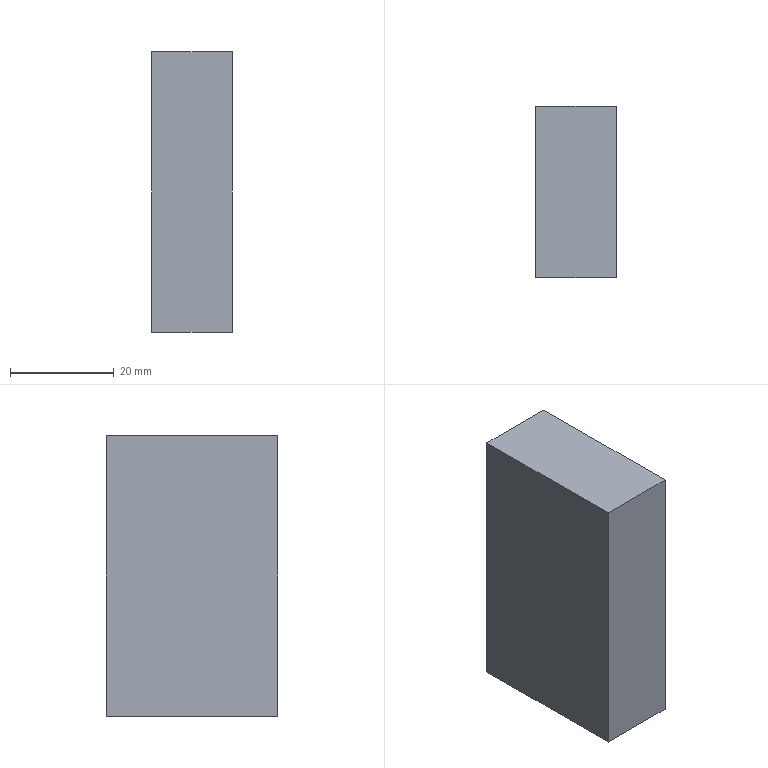Part | NX | features DATUM_CSYS 2, BLOCK 1, EXTRUDE 1, SKETCH 1 | 1 solid | 8 faces | box 15.5 x 33 x 54 mm | volume 25530 mm3 | plane 7 | cylinder 1 | commonest cylinder face diameters 22 x1
STEP:
#1=CARTESIAN_POINT('',(15.5,0.,54.));
#2=VERTEX_POINT('',#1);
#3=CARTESIAN_POINT('',(0.,0.,54.));
#4=VERTEX_POINT('',#3);
#5=CARTESIAN_POINT('',(7.75,0.,54.));
#6=DIRECTION('',(-1.,0.,0.));
#7=VECTOR('',#6,1000.);
#8=LINE('',#5,#7);
#9=EDGE_CURVE('',#2,#4,#8,.T.);
#10=ORIENTED_EDGE('',*,*,#9,.F.);
#11=CARTESIAN_POINT('',(15.5,33.,54.));
#12=VERTEX_POINT('',#11);
#13=CARTESIAN_POINT('',(15.5,16.5,54.));
#14=DIRECTION('',(0.,-1.,0.));
#15=VECTOR('',#14,1000.);
#16=LINE('',#13,#15);
#17=EDGE_CURVE('',#12,#2,#16,.T.);
#18=ORIENTED_EDGE('',*,*,#17,.F.);
#19=CARTESIAN_POINT('',(0.,33.,54.));
#20=VERTEX_POINT('',#19);
#21=CARTESIAN_POINT('',(7.75,33.,54.));
#22=DIRECTION('',(1.,0.,0.));
#23=VECTOR('',#22,1000.);
#24=LINE('',#21,#23);
#25=EDGE_CURVE('',#20,#12,#24,.T.);
#26=ORIENTED_EDGE('',*,*,#25,.F.);
#27=CARTESIAN_POINT('',(0.,16.5,54.));
#28=DIRECTION('',(0.,1.,0.));
#29=VECTOR('',#28,1000.);
#30=LINE('',#27,#29);
#31=EDGE_CURVE('',#4,#20,#30,.T.);
#32=ORIENTED_EDGE('',*,*,#31,.F.);
#33=EDGE_LOOP('',(#10,#18,#26,#32));
#34=FACE_BOUND('',#33,.T.);
#35=CARTESIAN_POINT('',(7.75,16.5,54.));
#36=DIRECTION('',(0.,0.,1.));
#37=DIRECTION('',(1.,0.,0.));
#38=AXIS2_PLACEMENT_3D('',#35,#36,#37);
#39=PLANE('',#38);
#40=ADVANCED_FACE('',(#34),#39,.T.);
#41=CARTESIAN_POINT('',(15.5,0.,0.));
#42=VERTEX_POINT('',#41);
#43=CARTESIAN_POINT('',(15.5,0.,0.));
#44=DIRECTION('',(0.,0.,1.));
#45=VECTOR('',#44,1000.);
#46=LINE('',#43,#45);
#47=EDGE_CURVE('',#42,#2,#46,.T.);
#48=ORIENTED_EDGE('',*,*,#47,.T.);
#49=ORIENTED_EDGE('',*,*,#9,.T.);
#50=CARTESIAN_POINT('',(0.,0.,0.));
#51=VERTEX_POINT('',#50);
#52=CARTESIAN_POINT('',(0.,0.,0.));
#53=DIRECTION('',(0.,0.,1.));
#54=VECTOR('',#53,1000.);
#55=LINE('',#52,#54);
#56=EDGE_CURVE('',#51,#4,#55,.T.);
#57=ORIENTED_EDGE('',*,*,#56,.F.);
#58=CARTESIAN_POINT('',(7.75,0.,0.));
#59=DIRECTION('',(1.,0.,0.));
#60=VECTOR('',#59,1000.);
#61=LINE('',#58,#60);
#62=EDGE_CURVE('',#51,#42,#61,.T.);
#63=ORIENTED_EDGE('',*,*,#62,.T.);
#64=EDGE_LOOP('',(#48,#49,#57,#63));
#65=FACE_BOUND('',#64,.T.);
#66=CARTESIAN_POINT('',(7.75,0.,0.));
#67=DIRECTION('',(0.,-1.,0.));
#68=DIRECTION('',(0.,0.,-1.));
#69=AXIS2_PLACEMENT_3D('',#66,#67,#68);
#70=PLANE('',#69);
#71=ADVANCED_FACE('',(#65),#70,.T.);
#72=ORIENTED_EDGE('',*,*,#56,.T.);
#73=ORIENTED_EDGE('',*,*,#31,.T.);
#74=CARTESIAN_POINT('',(0.,33.,0.));
#75=VERTEX_POINT('',#74);
#76=CARTESIAN_POINT('',(0.,33.,0.));
#77=DIRECTION('',(0.,0.,1.));
#78=VECTOR('',#77,1000.);
#79=LINE('',#76,#78);
#80=EDGE_CURVE('',#75,#20,#79,.T.);
#81=ORIENTED_EDGE('',*,*,#80,.F.);
#82=CARTESIAN_POINT('',(0.,16.5,0.));
#83=DIRECTION('',(0.,-1.,0.));
#84=VECTOR('',#83,1000.);
#85=LINE('',#82,#84);
#86=EDGE_CURVE('',#75,#51,#85,.T.);
#87=ORIENTED_EDGE('',*,*,#86,.T.);
#88=EDGE_LOOP('',(#72,#73,#81,#87));
#89=FACE_BOUND('',#88,.T.);
#90=CARTESIAN_POINT('',(0.,16.5,0.));
#91=DIRECTION('',(-1.,0.,0.));
#92=DIRECTION('',(0.,0.,1.));
#93=AXIS2_PLACEMENT_3D('',#90,#91,#92);
#94=PLANE('',#93);
#95=ADVANCED_FACE('',(#89),#94,.T.);
#96=ORIENTED_EDGE('',*,*,#80,.T.);
#97=ORIENTED_EDGE('',*,*,#25,.T.);
#98=CARTESIAN_POINT('',(15.5,33.,0.));
#99=VERTEX_POINT('',#98);
#100=CARTESIAN_POINT('',(15.5,33.,0.));
#101=DIRECTION('',(0.,0.,1.));
#102=VECTOR('',#101,1000.);
#103=LINE('',#100,#102);
#104=EDGE_CURVE('',#99,#12,#103,.T.);
#105=ORIENTED_EDGE('',*,*,#104,.F.);
#106=CARTESIAN_POINT('',(7.75,33.,0.));
#107=DIRECTION('',(-1.,0.,0.));
#108=VECTOR('',#107,1000.);
#109=LINE('',#106,#108);
#110=EDGE_CURVE('',#99,#75,#109,.T.);
#111=ORIENTED_EDGE('',*,*,#110,.T.);
#112=EDGE_LOOP('',(#96,#97,#105,#111));
#113=FACE_BOUND('',#112,.T.);
#114=CARTESIAN_POINT('',(7.75,33.,0.));
#115=DIRECTION('',(0.,1.,0.));
#116=DIRECTION('',(0.,0.,1.));
#117=AXIS2_PLACEMENT_3D('',#114,#115,#116);
#118=PLANE('',#117);
#119=ADVANCED_FACE('',(#113),#118,.T.);
#120=CARTESIAN_POINT('',(15.5,16.5,0.));
#121=DIRECTION('',(0.,1.,0.));
#122=VECTOR('',#121,1000.);
#123=LINE('',#120,#122);
#124=EDGE_CURVE('',#42,#99,#123,.T.);
#125=ORIENTED_EDGE('',*,*,#124,.F.);
#126=ORIENTED_EDGE('',*,*,#62,.F.);
#127=ORIENTED_EDGE('',*,*,#86,.F.);
#128=ORIENTED_EDGE('',*,*,#110,.F.);
#129=EDGE_LOOP('',(#125,#126,#127,#128));
#130=FACE_BOUND('',#129,.T.);
#131=CARTESIAN_POINT('',(7.75,16.5,0.));
#132=DIRECTION('',(0.,0.,-1.));
#133=DIRECTION('',(-1.,0.,0.));
#134=AXIS2_PLACEMENT_3D('',#131,#132,#133);
#135=PLANE('',#134);
#136=ADVANCED_FACE('',(#130),#135,.T.);
#137=CARTESIAN_POINT('',(15.5,30.,27.));
#138=VERTEX_POINT('',#137);
#139=CARTESIAN_POINT('',(15.5,19.,27.));
#140=DIRECTION('',(1.,0.,0.));
#141=DIRECTION('',(0.,1.,0.));
#142=AXIS2_PLACEMENT_3D('',#139,#140,#141);
#143=CIRCLE('',#142,11.);
#144=EDGE_CURVE('',#138,#138,#143,.T.);
#145=ORIENTED_EDGE('',*,*,#144,.F.);
#146=EDGE_LOOP('',(#145));
#147=FACE_BOUND('',#146,.T.);
#148=ORIENTED_EDGE('',*,*,#124,.T.);
#149=ORIENTED_EDGE('',*,*,#104,.T.);
#150=ORIENTED_EDGE('',*,*,#17,.T.);
#151=ORIENTED_EDGE('',*,*,#47,.F.);
#152=EDGE_LOOP('',(#148,#149,#150,#151));
#153=FACE_BOUND('',#152,.T.);
#154=CARTESIAN_POINT('',(15.5,16.5,0.));
#155=DIRECTION('',(1.,0.,0.));
#156=DIRECTION('',(0.,0.,-1.));
#157=AXIS2_PLACEMENT_3D('',#154,#155,#156);
#158=PLANE('',#157);
#159=ADVANCED_FACE('',(#147,#153),#158,.T.);
#160=CARTESIAN_POINT('',(10.,30.,27.));
#161=VERTEX_POINT('',#160);
#162=CARTESIAN_POINT('',(10.,19.,27.));
#163=DIRECTION('',(1.,0.,0.));
#164=DIRECTION('',(0.,1.,0.));
#165=AXIS2_PLACEMENT_3D('',#162,#163,#164);
#166=CIRCLE('',#165,11.);
#167=EDGE_CURVE('',#161,#161,#166,.F.);
#168=ORIENTED_EDGE('',*,*,#167,.T.);
#169=EDGE_LOOP('',(#168));
#170=FACE_BOUND('',#169,.T.);
#171=ORIENTED_EDGE('',*,*,#144,.T.);
#172=EDGE_LOOP('',(#171));
#173=FACE_BOUND('',#172,.T.);
#174=CARTESIAN_POINT('',(10.,19.,27.));
#175=DIRECTION('',(1.,0.,0.));
#176=DIRECTION('',(0.,0.,-1.));
#177=AXIS2_PLACEMENT_3D('',#174,#175,#176);
#178=CYLINDRICAL_SURFACE('',#177,11.);
#179=ADVANCED_FACE('',(#170,#173),#178,.F.);
#180=ORIENTED_EDGE('',*,*,#167,.F.);
#181=EDGE_LOOP('',(#180));
#182=FACE_BOUND('',#181,.T.);
#183=CARTESIAN_POINT('',(10.,19.,27.));
#184=DIRECTION('',(1.,0.,0.));
#185=DIRECTION('',(0.,0.,-1.));
#186=AXIS2_PLACEMENT_3D('',#183,#184,#185);
#187=PLANE('',#186);
#188=ADVANCED_FACE('',(#182),#187,.T.);
#189=CLOSED_SHELL('',(#40,#71,#95,#119,#136,#159,#179,#188));
#190=MANIFOLD_SOLID_BREP('',#189);
#191=(LENGTH_UNIT()NAMED_UNIT(*)SI_UNIT(.MILLI.,.METRE.));
#192=UNCERTAINTY_MEASURE_WITH_UNIT(LENGTH_MEASURE(0.00001),#191,'','');
#193=(NAMED_UNIT(*)PLANE_ANGLE_UNIT()SI_UNIT($,.RADIAN.));
#194=(NAMED_UNIT(*)SI_UNIT($,.STERADIAN.)SOLID_ANGLE_UNIT());
#195=(GEOMETRIC_REPRESENTATION_CONTEXT(3)GLOBAL_UNCERTAINTY_ASSIGNED_CONTEXT((#192))GLOBAL_UNIT_ASSIGNED_CONTEXT((#191,#193,#194))REPRESENTATION_CONTEXT('',''));
#196=ADVANCED_BREP_SHAPE_REPRESENTATION('',(#190),#195);